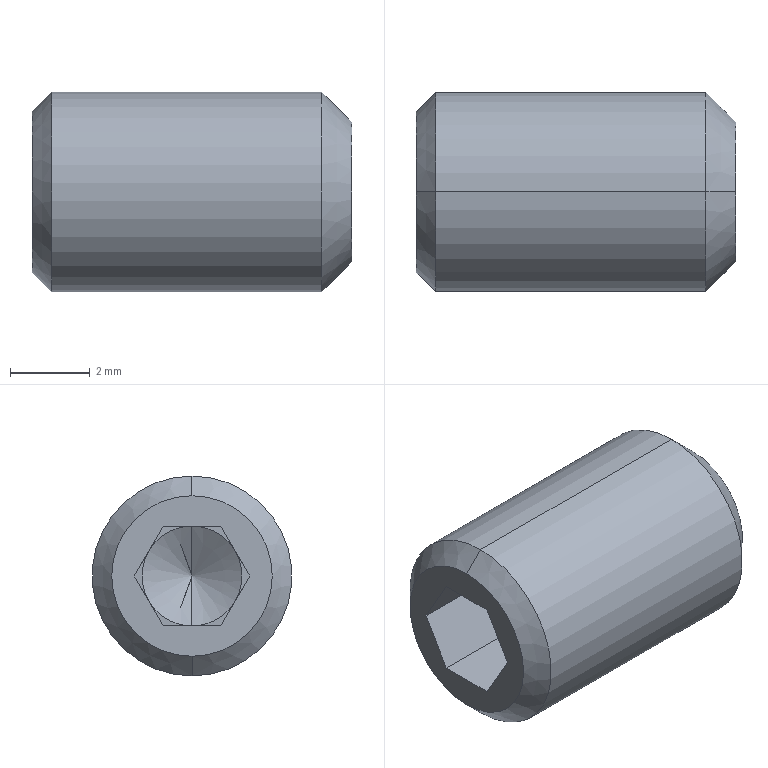Part | STEP file | 0228_305_MSSFS5-8 | 1 solid | 22 faces | box 8 x 5 x 5 mm | volume 139.331 mm3 | plane 14 | cone 6 | cylinder 2 | commonest cylinder face diameters 5 x2
STEP:
#1=CARTESIAN_POINT('',(0.,0.,0.));
#2=DIRECTION('',(0.,0.,1.));
#3=DIRECTION('',(1.,0.,0.));
#4=AXIS2_PLACEMENT_3D('',#1,#2,#3);
#5=CARTESIAN_POINT('',(-3.51,0.,-2.5));
#6=VERTEX_POINT('',#5);
#7=CARTESIAN_POINT('',(-3.51,0.,2.5));
#8=VERTEX_POINT('',#7);
#9=CARTESIAN_POINT('',(-3.51,0.,0.));
#10=DIRECTION('',(1.,0.,0.));
#11=DIRECTION('',(0.,0.,-1.));
#12=AXIS2_PLACEMENT_3D('',#9,#10,#11);
#13=CIRCLE('',#12,2.5);
#14=CARTESIAN_POINT('',(-0.1298,0.,0.));
#15=DIRECTION('',(1.,0.,0.));
#16=DIRECTION('',(0.,0.,-1.));
#17=AXIS2_PLACEMENT_3D('',#14,#15,#16);
#18=CYLINDRICAL_SURFACE('',#17,2.5);
#19=CARTESIAN_POINT('',(0.,-3.38));
#20=DIRECTION('',(1.,0.));
#21=VECTOR('',#20,1.);
#22=LINE('',#19,#21);
#23=(GEOMETRIC_REPRESENTATION_CONTEXT(2)PARAMETRIC_REPRESENTATION_CONTEXT()REPRESENTATION_CONTEXT('',''));
#24=DEFINITIONAL_REPRESENTATION('',(#22),#23);
#25=PCURVE('',#18,#24);
#26=CARTESIAN_POINT('',(-3.51,0.,0.));
#27=DIRECTION('',(1.,0.,0.));
#28=DIRECTION('',(0.,0.,-1.));
#29=AXIS2_PLACEMENT_3D('',#26,#27,#28);
#30=CONICAL_SURFACE('',#29,2.5,0.7854);
#31=CARTESIAN_POINT('',(0.,0.));
#32=DIRECTION('',(1.,0.));
#33=VECTOR('',#32,1.);
#34=LINE('',#31,#33);
#35=(GEOMETRIC_REPRESENTATION_CONTEXT(2)PARAMETRIC_REPRESENTATION_CONTEXT()REPRESENTATION_CONTEXT('',''));
#36=DEFINITIONAL_REPRESENTATION('',(#34),#35);
#37=PCURVE('',#30,#36);
#38=SURFACE_CURVE('',#13,(#25,#37),.PCURVE_S1.);
#39=EDGE_CURVE('',#6,#8,#38,.T.);
#40=ORIENTED_EDGE('',*,*,#39,.T.);
#41=CARTESIAN_POINT('',(3.25,0.,2.5));
#42=VERTEX_POINT('',#41);
#43=CARTESIAN_POINT('',(-0.1298,0.,2.5));
#44=DIRECTION('',(1.,0.,0.));
#45=VECTOR('',#44,1.);
#46=LINE('',#43,#45);
#47=CARTESIAN_POINT('',(3.142,0.));
#48=DIRECTION('',(0.,1.));
#49=VECTOR('',#48,1.);
#50=LINE('',#47,#49);
#51=(GEOMETRIC_REPRESENTATION_CONTEXT(2)PARAMETRIC_REPRESENTATION_CONTEXT()REPRESENTATION_CONTEXT('',''));
#52=DEFINITIONAL_REPRESENTATION('',(#50),#51);
#53=PCURVE('',#18,#52);
#54=CARTESIAN_POINT('',(-0.1298,0.,0.));
#55=DIRECTION('',(1.,0.,0.));
#56=DIRECTION('',(0.,0.,-1.));
#57=AXIS2_PLACEMENT_3D('',#54,#55,#56);
#58=CYLINDRICAL_SURFACE('',#57,2.5);
#59=CARTESIAN_POINT('',(3.142,0.));
#60=DIRECTION('',(0.,1.));
#61=VECTOR('',#60,1.);
#62=LINE('',#59,#61);
#63=(GEOMETRIC_REPRESENTATION_CONTEXT(2)PARAMETRIC_REPRESENTATION_CONTEXT()REPRESENTATION_CONTEXT('',''));
#64=DEFINITIONAL_REPRESENTATION('',(#62),#63);
#65=PCURVE('',#58,#64);
#66=SURFACE_CURVE('',#46,(#53,#65),.PCURVE_S1.);
#67=EDGE_CURVE('',#8,#42,#66,.T.);
#68=ORIENTED_EDGE('',*,*,#67,.T.);
#69=CARTESIAN_POINT('',(3.25,0.,-2.5));
#70=VERTEX_POINT('',#69);
#71=CARTESIAN_POINT('',(3.25,0.,0.));
#72=DIRECTION('',(-1.,0.,0.));
#73=DIRECTION('',(0.,0.,-1.));
#74=AXIS2_PLACEMENT_3D('',#71,#72,#73);
#75=CIRCLE('',#74,2.5);
#76=CARTESIAN_POINT('',(6.283,3.38));
#77=DIRECTION('',(-1.,0.));
#78=VECTOR('',#77,1.);
#79=LINE('',#76,#78);
#80=(GEOMETRIC_REPRESENTATION_CONTEXT(2)PARAMETRIC_REPRESENTATION_CONTEXT()REPRESENTATION_CONTEXT('',''));
#81=DEFINITIONAL_REPRESENTATION('',(#79),#80);
#82=PCURVE('',#18,#81);
#83=CARTESIAN_POINT('',(3.25,0.,0.));
#84=DIRECTION('',(-1.,0.,0.));
#85=DIRECTION('',(0.,0.,1.));
#86=AXIS2_PLACEMENT_3D('',#83,#84,#85);
#87=CONICAL_SURFACE('',#86,2.5,0.7854);
#88=CARTESIAN_POINT('',(-3.142,0.));
#89=DIRECTION('',(1.,0.));
#90=VECTOR('',#89,1.);
#91=LINE('',#88,#90);
#92=(GEOMETRIC_REPRESENTATION_CONTEXT(2)PARAMETRIC_REPRESENTATION_CONTEXT()REPRESENTATION_CONTEXT('',''));
#93=DEFINITIONAL_REPRESENTATION('',(#91),#92);
#94=PCURVE('',#87,#93);
#95=SURFACE_CURVE('',#75,(#82,#94),.PCURVE_S1.);
#96=EDGE_CURVE('',#42,#70,#95,.T.);
#97=ORIENTED_EDGE('',*,*,#96,.T.);
#98=CARTESIAN_POINT('',(-0.1298,0.,-2.5));
#99=DIRECTION('',(1.,0.,0.));
#100=VECTOR('',#99,1.);
#101=LINE('',#98,#100);
#102=CARTESIAN_POINT('',(0.,0.));
#103=DIRECTION('',(0.,1.));
#104=VECTOR('',#103,1.);
#105=LINE('',#102,#104);
#106=(GEOMETRIC_REPRESENTATION_CONTEXT(2)PARAMETRIC_REPRESENTATION_CONTEXT()REPRESENTATION_CONTEXT('',''));
#107=DEFINITIONAL_REPRESENTATION('',(#105),#106);
#108=PCURVE('',#18,#107);
#109=CARTESIAN_POINT('',(6.283,0.));
#110=DIRECTION('',(0.,1.));
#111=VECTOR('',#110,1.);
#112=LINE('',#109,#111);
#113=(GEOMETRIC_REPRESENTATION_CONTEXT(2)PARAMETRIC_REPRESENTATION_CONTEXT()REPRESENTATION_CONTEXT('',''));
#114=DEFINITIONAL_REPRESENTATION('',(#112),#113);
#115=PCURVE('',#58,#114);
#116=SURFACE_CURVE('',#101,(#108,#115),.PCURVE_S1.);
#117=EDGE_CURVE('',#6,#70,#116,.T.);
#118=ORIENTED_EDGE('',*,*,#117,.F.);
#119=EDGE_LOOP('',(#40,#68,#97,#118));
#120=FACE_BOUND('',#119,.T.);
#121=ADVANCED_FACE('',(#120),#18,.T.);
#122=CARTESIAN_POINT('',(-4.,0.,-2.009));
#123=VERTEX_POINT('',#122);
#124=CARTESIAN_POINT('',(-4.,0.,2.009));
#125=VERTEX_POINT('',#124);
#126=CARTESIAN_POINT('',(-4.,0.,0.));
#127=DIRECTION('',(1.,0.,0.));
#128=DIRECTION('',(0.,0.,-1.));
#129=AXIS2_PLACEMENT_3D('',#126,#127,#128);
#130=CIRCLE('',#129,2.009);
#131=CARTESIAN_POINT('',(0.,-0.4905));
#132=DIRECTION('',(1.,0.));
#133=VECTOR('',#132,1.);
#134=LINE('',#131,#133);
#135=(GEOMETRIC_REPRESENTATION_CONTEXT(2)PARAMETRIC_REPRESENTATION_CONTEXT()REPRESENTATION_CONTEXT('',''));
#136=DEFINITIONAL_REPRESENTATION('',(#134),#135);
#137=PCURVE('',#30,#136);
#138=CARTESIAN_POINT('',(-4.,1.005,0.));
#139=DIRECTION('',(-1.,0.,0.));
#140=DIRECTION('',(0.,0.,1.));
#141=AXIS2_PLACEMENT_3D('',#138,#139,#140);
#142=PLANE('',#141);
#143=CARTESIAN_POINT('',(-2.009,-1.005));
#144=CARTESIAN_POINT('',(-2.009,2.476));
#145=CARTESIAN_POINT('',(1.005,0.7355));
#146=CARTESIAN_POINT('',(4.019,-1.005));
#147=CARTESIAN_POINT('',(1.005,-2.745));
#148=CARTESIAN_POINT('',(-2.009,-4.485));
#149=CARTESIAN_POINT('',(-2.009,-1.005));
#150=(BOUNDED_CURVE()B_SPLINE_CURVE(2,(#143,#144,#145,#146,#147,#148,#149),.UNSPECIFIED.,.T.,.F.)B_SPLINE_CURVE_WITH_KNOTS((1,2,2,2,2,1),(-2.094,0.,2.094,4.189,6.283,8.378),.UNSPECIFIED.)CURVE()GEOMETRIC_REPRESENTATION_ITEM()RATIONAL_B_SPLINE_CURVE((1.,0.5,1.,0.5,1.,0.5,1.))REPRESENTATION_ITEM(''));
#151=(GEOMETRIC_REPRESENTATION_CONTEXT(2)PARAMETRIC_REPRESENTATION_CONTEXT()REPRESENTATION_CONTEXT('',''));
#152=DEFINITIONAL_REPRESENTATION('',(#150),#151);
#153=PCURVE('',#142,#152);
#154=SURFACE_CURVE('',#130,(#137,#153),.PCURVE_S1.);
#155=EDGE_CURVE('',#123,#125,#154,.T.);
#156=ORIENTED_EDGE('',*,*,#155,.T.);
#157=CARTESIAN_POINT('',(-3.51,0.,2.5));
#158=DIRECTION('',(0.7071,0.,0.7071));
#159=VECTOR('',#158,1.);
#160=LINE('',#157,#159);
#161=CARTESIAN_POINT('',(3.142,0.));
#162=DIRECTION('',(0.,1.));
#163=VECTOR('',#162,1.);
#164=LINE('',#161,#163);
#165=(GEOMETRIC_REPRESENTATION_CONTEXT(2)PARAMETRIC_REPRESENTATION_CONTEXT()REPRESENTATION_CONTEXT('',''));
#166=DEFINITIONAL_REPRESENTATION('',(#164),#165);
#167=PCURVE('',#30,#166);
#168=CARTESIAN_POINT('',(-3.51,0.,0.));
#169=DIRECTION('',(1.,0.,0.));
#170=DIRECTION('',(0.,0.,-1.));
#171=AXIS2_PLACEMENT_3D('',#168,#169,#170);
#172=CONICAL_SURFACE('',#171,2.5,0.7854);
#173=CARTESIAN_POINT('',(3.142,0.));
#174=DIRECTION('',(0.,1.));
#175=VECTOR('',#174,1.);
#176=LINE('',#173,#175);
#177=(GEOMETRIC_REPRESENTATION_CONTEXT(2)PARAMETRIC_REPRESENTATION_CONTEXT()REPRESENTATION_CONTEXT('',''));
#178=DEFINITIONAL_REPRESENTATION('',(#176),#177);
#179=PCURVE('',#172,#178);
#180=SURFACE_CURVE('',#160,(#167,#179),.PCURVE_S1.);
#181=EDGE_CURVE('',#125,#8,#180,.T.);
#182=ORIENTED_EDGE('',*,*,#181,.T.);
#183=ORIENTED_EDGE('',*,*,#39,.F.);
#184=CARTESIAN_POINT('',(-3.51,0.,-2.5));
#185=DIRECTION('',(0.7071,0.,-0.7071));
#186=VECTOR('',#185,1.);
#187=LINE('',#184,#186);
#188=CARTESIAN_POINT('',(0.,0.));
#189=DIRECTION('',(0.,1.));
#190=VECTOR('',#189,1.);
#191=LINE('',#188,#190);
#192=(GEOMETRIC_REPRESENTATION_CONTEXT(2)PARAMETRIC_REPRESENTATION_CONTEXT()REPRESENTATION_CONTEXT('',''));
#193=DEFINITIONAL_REPRESENTATION('',(#191),#192);
#194=PCURVE('',#30,#193);
#195=CARTESIAN_POINT('',(6.283,0.));
#196=DIRECTION('',(0.,1.));
#197=VECTOR('',#196,1.);
#198=LINE('',#195,#197);
#199=(GEOMETRIC_REPRESENTATION_CONTEXT(2)PARAMETRIC_REPRESENTATION_CONTEXT()REPRESENTATION_CONTEXT('',''));
#200=DEFINITIONAL_REPRESENTATION('',(#198),#199);
#201=PCURVE('',#172,#200);
#202=SURFACE_CURVE('',#187,(#194,#201),.PCURVE_S1.);
#203=EDGE_CURVE('',#123,#6,#202,.T.);
#204=ORIENTED_EDGE('',*,*,#203,.F.);
#205=EDGE_LOOP('',(#156,#182,#183,#204));
#206=FACE_BOUND('',#205,.T.);
#207=ADVANCED_FACE('',(#206),#30,.T.);
#208=CARTESIAN_POINT('',(4.,0.,1.75));
#209=VERTEX_POINT('',#208);
#210=CARTESIAN_POINT('',(4.,0.,-1.75));
#211=VERTEX_POINT('',#210);
#212=CARTESIAN_POINT('',(4.,0.,0.));
#213=DIRECTION('',(-1.,0.,0.));
#214=DIRECTION('',(0.,0.,1.));
#215=AXIS2_PLACEMENT_3D('',#212,#213,#214);
#216=CIRCLE('',#215,1.75);
#217=CARTESIAN_POINT('',(0.,-0.75));
#218=DIRECTION('',(1.,0.));
#219=VECTOR('',#218,1.);
#220=LINE('',#217,#219);
#221=(GEOMETRIC_REPRESENTATION_CONTEXT(2)PARAMETRIC_REPRESENTATION_CONTEXT()REPRESENTATION_CONTEXT('',''));
#222=DEFINITIONAL_REPRESENTATION('',(#220),#221);
#223=PCURVE('',#87,#222);
#224=CARTESIAN_POINT('',(4.,0.875,0.));
#225=DIRECTION('',(1.,0.,0.));
#226=DIRECTION('',(0.,0.,-1.));
#227=AXIS2_PLACEMENT_3D('',#224,#225,#226);
#228=PLANE('',#227);
#229=CARTESIAN_POINT('',(-1.75,-0.875));
#230=CARTESIAN_POINT('',(-1.75,2.156));
#231=CARTESIAN_POINT('',(0.875,0.6405));
#232=CARTESIAN_POINT('',(3.5,-0.875));
#233=CARTESIAN_POINT('',(0.875,-2.391));
#234=CARTESIAN_POINT('',(-1.75,-3.906));
#235=CARTESIAN_POINT('',(-1.75,-0.875));
#236=(BOUNDED_CURVE()B_SPLINE_CURVE(2,(#229,#230,#231,#232,#233,#234,#235),.UNSPECIFIED.,.T.,.F.)B_SPLINE_CURVE_WITH_KNOTS((1,2,2,2,2,1),(-2.094,0.,2.094,4.189,6.283,8.378),.UNSPECIFIED.)CURVE()GEOMETRIC_REPRESENTATION_ITEM()RATIONAL_B_SPLINE_CURVE((1.,0.5,1.,0.5,1.,0.5,1.))REPRESENTATION_ITEM(''));
#237=(GEOMETRIC_REPRESENTATION_CONTEXT(2)PARAMETRIC_REPRESENTATION_CONTEXT()REPRESENTATION_CONTEXT('',''));
#238=DEFINITIONAL_REPRESENTATION('',(#236),#237);
#239=PCURVE('',#228,#238);
#240=SURFACE_CURVE('',#216,(#223,#239),.PCURVE_S1.);
#241=EDGE_CURVE('',#209,#211,#240,.T.);
#242=ORIENTED_EDGE('',*,*,#241,.T.);
#243=CARTESIAN_POINT('',(3.25,0.,-2.5));
#244=DIRECTION('',(-0.7071,0.,-0.7071));
#245=VECTOR('',#244,1.);
#246=LINE('',#243,#245);
#247=CARTESIAN_POINT('',(3.142,0.));
#248=DIRECTION('',(0.,1.));
#249=VECTOR('',#248,1.);
#250=LINE('',#247,#249);
#251=(GEOMETRIC_REPRESENTATION_CONTEXT(2)PARAMETRIC_REPRESENTATION_CONTEXT()REPRESENTATION_CONTEXT('',''));
#252=DEFINITIONAL_REPRESENTATION('',(#250),#251);
#253=PCURVE('',#87,#252);
#254=CARTESIAN_POINT('',(3.25,0.,0.));
#255=DIRECTION('',(-1.,0.,0.));
#256=DIRECTION('',(0.,0.,1.));
#257=AXIS2_PLACEMENT_3D('',#254,#255,#256);
#258=CONICAL_SURFACE('',#257,2.5,0.7854);
#259=CARTESIAN_POINT('',(3.142,0.));
#260=DIRECTION('',(0.,1.));
#261=VECTOR('',#260,1.);
#262=LINE('',#259,#261);
#263=(GEOMETRIC_REPRESENTATION_CONTEXT(2)PARAMETRIC_REPRESENTATION_CONTEXT()REPRESENTATION_CONTEXT('',''));
#264=DEFINITIONAL_REPRESENTATION('',(#262),#263);
#265=PCURVE('',#258,#264);
#266=SURFACE_CURVE('',#246,(#253,#265),.PCURVE_S1.);
#267=EDGE_CURVE('',#211,#70,#266,.T.);
#268=ORIENTED_EDGE('',*,*,#267,.T.);
#269=ORIENTED_EDGE('',*,*,#96,.F.);
#270=CARTESIAN_POINT('',(3.25,0.,2.5));
#271=DIRECTION('',(-0.7071,0.,0.7071));
#272=VECTOR('',#271,1.);
#273=LINE('',#270,#272);
#274=CARTESIAN_POINT('',(0.,0.));
#275=DIRECTION('',(0.,1.));
#276=VECTOR('',#275,1.);
#277=LINE('',#274,#276);
#278=(GEOMETRIC_REPRESENTATION_CONTEXT(2)PARAMETRIC_REPRESENTATION_CONTEXT()REPRESENTATION_CONTEXT('',''));
#279=DEFINITIONAL_REPRESENTATION('',(#277),#278);
#280=PCURVE('',#87,#279);
#281=CARTESIAN_POINT('',(6.283,0.));
#282=DIRECTION('',(0.,1.));
#283=VECTOR('',#282,1.);
#284=LINE('',#281,#283);
#285=(GEOMETRIC_REPRESENTATION_CONTEXT(2)PARAMETRIC_REPRESENTATION_CONTEXT()REPRESENTATION_CONTEXT('',''));
#286=DEFINITIONAL_REPRESENTATION('',(#284),#285);
#287=PCURVE('',#258,#286);
#288=SURFACE_CURVE('',#273,(#280,#287),.PCURVE_S1.);
#289=EDGE_CURVE('',#209,#42,#288,.T.);
#290=ORIENTED_EDGE('',*,*,#289,.F.);
#291=EDGE_LOOP('',(#242,#268,#269,#290));
#292=FACE_BOUND('',#291,.T.);
#293=ADVANCED_FACE('',(#292),#87,.T.);
#294=CARTESIAN_POINT('',(-2.,0.,1.25));
#295=VERTEX_POINT('',#294);
#296=CARTESIAN_POINT('',(-2.,-1.083,0.625));
#297=VERTEX_POINT('',#296);
#298=CARTESIAN_POINT('',(-2.,0.,0.));
#299=DIRECTION('',(1.,0.,0.));
#300=DIRECTION('',(0.,0.,1.));
#301=AXIS2_PLACEMENT_3D('',#298,#299,#300);
#302=CIRCLE('',#301,1.25);
#303=CARTESIAN_POINT('',(-2.,0.,0.));
#304=DIRECTION('',(-1.,0.,0.));
#305=DIRECTION('',(0.,0.,1.));
#306=AXIS2_PLACEMENT_3D('',#303,#304,#305);
#307=CONICAL_SURFACE('',#306,1.25,1.047);
#308=CARTESIAN_POINT('',(6.283,0.));
#309=DIRECTION('',(-1.,0.));
#310=VECTOR('',#309,1.);
#311=LINE('',#308,#310);
#312=(GEOMETRIC_REPRESENTATION_CONTEXT(2)PARAMETRIC_REPRESENTATION_CONTEXT()REPRESENTATION_CONTEXT('',''));
#313=DEFINITIONAL_REPRESENTATION('',(#311),#312);
#314=PCURVE('',#307,#313);
#315=CARTESIAN_POINT('',(-2.,0.,0.));
#316=DIRECTION('',(1.,0.,0.));
#317=DIRECTION('',(0.,0.,-1.));
#318=AXIS2_PLACEMENT_3D('',#315,#316,#317);
#319=PLANE('',#318);
#320=CARTESIAN_POINT('',(0.,0.));
#321=DIRECTION('',(-1.,0.));
#322=AXIS2_PLACEMENT_2D('',#320,#321);
#323=CIRCLE('',#322,1.25);
#324=(GEOMETRIC_REPRESENTATION_CONTEXT(2)PARAMETRIC_REPRESENTATION_CONTEXT()REPRESENTATION_CONTEXT('',''));
#325=DEFINITIONAL_REPRESENTATION('',(#323),#324);
#326=PCURVE('',#319,#325);
#327=SURFACE_CURVE('',#302,(#314,#326),.PCURVE_S1.);
#328=EDGE_CURVE('',#295,#297,#327,.T.);
#329=ORIENTED_EDGE('',*,*,#328,.T.);
#330=CARTESIAN_POINT('',(-2.,-1.083,-0.625));
#331=VERTEX_POINT('',#330);
#332=CARTESIAN_POINT('',(-2.,0.,0.));
#333=DIRECTION('',(1.,0.,0.));
#334=DIRECTION('',(0.,0.,1.));
#335=AXIS2_PLACEMENT_3D('',#332,#333,#334);
#336=CIRCLE('',#335,1.25);
#337=CARTESIAN_POINT('',(6.283,0.));
#338=DIRECTION('',(-1.,0.));
#339=VECTOR('',#338,1.);
#340=LINE('',#337,#339);
#341=(GEOMETRIC_REPRESENTATION_CONTEXT(2)PARAMETRIC_REPRESENTATION_CONTEXT()REPRESENTATION_CONTEXT('',''));
#342=DEFINITIONAL_REPRESENTATION('',(#340),#341);
#343=PCURVE('',#307,#342);
#344=CARTESIAN_POINT('',(-2.,0.,0.));
#345=DIRECTION('',(1.,0.,0.));
#346=DIRECTION('',(0.,0.,-1.));
#347=AXIS2_PLACEMENT_3D('',#344,#345,#346);
#348=PLANE('',#347);
#349=CARTESIAN_POINT('',(0.,0.));
#350=DIRECTION('',(-1.,0.));
#351=AXIS2_PLACEMENT_2D('',#349,#350);
#352=CIRCLE('',#351,1.25);
#353=(GEOMETRIC_REPRESENTATION_CONTEXT(2)PARAMETRIC_REPRESENTATION_CONTEXT()REPRESENTATION_CONTEXT('',''));
#354=DEFINITIONAL_REPRESENTATION('',(#352),#353);
#355=PCURVE('',#348,#354);
#356=SURFACE_CURVE('',#336,(#343,#355),.PCURVE_S1.);
#357=EDGE_CURVE('',#297,#331,#356,.T.);
#358=ORIENTED_EDGE('',*,*,#357,.T.);
#359=CARTESIAN_POINT('',(-2.,0.,-1.25));
#360=VERTEX_POINT('',#359);
#361=CARTESIAN_POINT('',(-2.,0.,0.));
#362=DIRECTION('',(-1.,0.,0.));
#363=DIRECTION('',(0.,0.,1.));
#364=AXIS2_PLACEMENT_3D('',#361,#362,#363);
#365=CIRCLE('',#364,1.25);
#366=CARTESIAN_POINT('',(0.,0.));
#367=DIRECTION('',(1.,0.));
#368=VECTOR('',#367,1.);
#369=LINE('',#366,#368);
#370=(GEOMETRIC_REPRESENTATION_CONTEXT(2)PARAMETRIC_REPRESENTATION_CONTEXT()REPRESENTATION_CONTEXT('',''));
#371=DEFINITIONAL_REPRESENTATION('',(#369),#370);
#372=PCURVE('',#307,#371);
#373=CARTESIAN_POINT('',(-2.,0.,0.));
#374=DIRECTION('',(1.,0.,0.));
#375=DIRECTION('',(0.,0.,-1.));
#376=AXIS2_PLACEMENT_3D('',#373,#374,#375);
#377=PLANE('',#376);
#378=CARTESIAN_POINT('',(-1.25,0.));
#379=CARTESIAN_POINT('',(-1.25,2.165));
#380=CARTESIAN_POINT('',(0.625,1.083));
#381=CARTESIAN_POINT('',(2.5,0.));
#382=CARTESIAN_POINT('',(0.625,-1.083));
#383=CARTESIAN_POINT('',(-1.25,-2.165));
#384=CARTESIAN_POINT('',(-1.25,0.));
#385=(BOUNDED_CURVE()B_SPLINE_CURVE(2,(#378,#379,#380,#381,#382,#383,#384),.UNSPECIFIED.,.T.,.F.)B_SPLINE_CURVE_WITH_KNOTS((1,2,2,2,2,1),(-2.094,0.,2.094,4.189,6.283,8.378),.UNSPECIFIED.)CURVE()GEOMETRIC_REPRESENTATION_ITEM()RATIONAL_B_SPLINE_CURVE((1.,0.5,1.,0.5,1.,0.5,1.))REPRESENTATION_ITEM(''));
#386=(GEOMETRIC_REPRESENTATION_CONTEXT(2)PARAMETRIC_REPRESENTATION_CONTEXT()REPRESENTATION_CONTEXT('',''));
#387=DEFINITIONAL_REPRESENTATION('',(#385),#386);
#388=PCURVE('',#377,#387);
#389=SURFACE_CURVE('',#365,(#372,#388),.PCURVE_S1.);
#390=EDGE_CURVE('',#360,#331,#389,.T.);
#391=ORIENTED_EDGE('',*,*,#390,.F.);
#392=CARTESIAN_POINT('',(-1.278,0.,0.));
#393=VERTEX_POINT('',#392);
#394=CARTESIAN_POINT('',(-2.,0.,-1.25));
#395=DIRECTION('',(-0.5,0.,-0.866));
#396=VECTOR('',#395,1.);
#397=LINE('',#394,#396);
#398=CARTESIAN_POINT('',(3.142,0.));
#399=DIRECTION('',(0.,1.));
#400=VECTOR('',#399,1.);
#401=LINE('',#398,#400);
#402=(GEOMETRIC_REPRESENTATION_CONTEXT(2)PARAMETRIC_REPRESENTATION_CONTEXT()REPRESENTATION_CONTEXT('',''));
#403=DEFINITIONAL_REPRESENTATION('',(#401),#402);
#404=PCURVE('',#307,#403);
#405=CARTESIAN_POINT('',(-2.,0.,0.));
#406=DIRECTION('',(-1.,0.,0.));
#407=DIRECTION('',(0.,0.,1.));
#408=AXIS2_PLACEMENT_3D('',#405,#406,#407);
#409=CONICAL_SURFACE('',#408,1.25,1.047);
#410=CARTESIAN_POINT('',(3.142,0.));
#411=DIRECTION('',(0.,1.));
#412=VECTOR('',#411,1.);
#413=LINE('',#410,#412);
#414=(GEOMETRIC_REPRESENTATION_CONTEXT(2)PARAMETRIC_REPRESENTATION_CONTEXT()REPRESENTATION_CONTEXT('',''));
#415=DEFINITIONAL_REPRESENTATION('',(#413),#414);
#416=PCURVE('',#409,#415);
#417=SURFACE_CURVE('',#397,(#404,#416),.PCURVE_S1.);
#418=EDGE_CURVE('',#393,#360,#417,.T.);
#419=ORIENTED_EDGE('',*,*,#418,.F.);
#420=CARTESIAN_POINT('',(-2.,0.,1.25));
#421=DIRECTION('',(-0.5,0.,0.866));
#422=VECTOR('',#421,1.);
#423=LINE('',#420,#422);
#424=CARTESIAN_POINT('',(6.283,0.));
#425=DIRECTION('',(0.,1.));
#426=VECTOR('',#425,1.);
#427=LINE('',#424,#426);
#428=(GEOMETRIC_REPRESENTATION_CONTEXT(2)PARAMETRIC_REPRESENTATION_CONTEXT()REPRESENTATION_CONTEXT('',''));
#429=DEFINITIONAL_REPRESENTATION('',(#427),#428);
#430=PCURVE('',#307,#429);
#431=CARTESIAN_POINT('',(0.,0.));
#432=DIRECTION('',(0.,1.));
#433=VECTOR('',#432,1.);
#434=LINE('',#431,#433);
#435=(GEOMETRIC_REPRESENTATION_CONTEXT(2)PARAMETRIC_REPRESENTATION_CONTEXT()REPRESENTATION_CONTEXT('',''));
#436=DEFINITIONAL_REPRESENTATION('',(#434),#435);
#437=PCURVE('',#409,#436);
#438=SURFACE_CURVE('',#423,(#430,#437),.PCURVE_S1.);
#439=EDGE_CURVE('',#393,#295,#438,.T.);
#440=ORIENTED_EDGE('',*,*,#439,.T.);
#441=EDGE_LOOP('',(#329,#358,#391,#419,#440));
#442=FACE_BOUND('',#441,.F.);
#443=ADVANCED_FACE('',(#442),#307,.F.);
#444=ORIENTED_EDGE('',*,*,#67,.F.);
#445=CARTESIAN_POINT('',(-3.51,0.,0.));
#446=DIRECTION('',(1.,0.,0.));
#447=DIRECTION('',(0.,0.,-1.));
#448=AXIS2_PLACEMENT_3D('',#445,#446,#447);
#449=CIRCLE('',#448,2.5);
#450=CARTESIAN_POINT('',(0.,-3.38));
#451=DIRECTION('',(1.,0.));
#452=VECTOR('',#451,1.);
#453=LINE('',#450,#452);
#454=(GEOMETRIC_REPRESENTATION_CONTEXT(2)PARAMETRIC_REPRESENTATION_CONTEXT()REPRESENTATION_CONTEXT('',''));
#455=DEFINITIONAL_REPRESENTATION('',(#453),#454);
#456=PCURVE('',#58,#455);
#457=CARTESIAN_POINT('',(0.,0.));
#458=DIRECTION('',(1.,0.));
#459=VECTOR('',#458,1.);
#460=LINE('',#457,#459);
#461=(GEOMETRIC_REPRESENTATION_CONTEXT(2)PARAMETRIC_REPRESENTATION_CONTEXT()REPRESENTATION_CONTEXT('',''));
#462=DEFINITIONAL_REPRESENTATION('',(#460),#461);
#463=PCURVE('',#172,#462);
#464=SURFACE_CURVE('',#449,(#456,#463),.PCURVE_S1.);
#465=EDGE_CURVE('',#8,#6,#464,.T.);
#466=ORIENTED_EDGE('',*,*,#465,.T.);
#467=ORIENTED_EDGE('',*,*,#117,.T.);
#468=CARTESIAN_POINT('',(3.25,0.,0.));
#469=DIRECTION('',(-1.,0.,0.));
#470=DIRECTION('',(0.,0.,-1.));
#471=AXIS2_PLACEMENT_3D('',#468,#469,#470);
#472=CIRCLE('',#471,2.5);
#473=CARTESIAN_POINT('',(6.283,3.38));
#474=DIRECTION('',(-1.,0.));
#475=VECTOR('',#474,1.);
#476=LINE('',#473,#475);
#477=(GEOMETRIC_REPRESENTATION_CONTEXT(2)PARAMETRIC_REPRESENTATION_CONTEXT()REPRESENTATION_CONTEXT('',''));
#478=DEFINITIONAL_REPRESENTATION('',(#476),#477);
#479=PCURVE('',#58,#478);
#480=CARTESIAN_POINT('',(3.142,0.));
#481=DIRECTION('',(1.,0.));
#482=VECTOR('',#481,1.);
#483=LINE('',#480,#482);
#484=(GEOMETRIC_REPRESENTATION_CONTEXT(2)PARAMETRIC_REPRESENTATION_CONTEXT()REPRESENTATION_CONTEXT('',''));
#485=DEFINITIONAL_REPRESENTATION('',(#483),#484);
#486=PCURVE('',#258,#485);
#487=SURFACE_CURVE('',#472,(#479,#486),.PCURVE_S1.);
#488=EDGE_CURVE('',#70,#42,#487,.T.);
#489=ORIENTED_EDGE('',*,*,#488,.T.);
#490=EDGE_LOOP('',(#444,#466,#467,#489));
#491=FACE_BOUND('',#490,.T.);
#492=ADVANCED_FACE('',(#491),#58,.T.);
#493=ORIENTED_EDGE('',*,*,#181,.F.);
#494=CARTESIAN_POINT('',(-4.,0.,0.));
#495=DIRECTION('',(1.,0.,0.));
#496=DIRECTION('',(0.,0.,-1.));
#497=AXIS2_PLACEMENT_3D('',#494,#495,#496);
#498=CIRCLE('',#497,2.009);
#499=CARTESIAN_POINT('',(0.,-0.4905));
#500=DIRECTION('',(1.,0.));
#501=VECTOR('',#500,1.);
#502=LINE('',#499,#501);
#503=(GEOMETRIC_REPRESENTATION_CONTEXT(2)PARAMETRIC_REPRESENTATION_CONTEXT()REPRESENTATION_CONTEXT('',''));
#504=DEFINITIONAL_REPRESENTATION('',(#502),#503);
#505=PCURVE('',#172,#504);
#506=CARTESIAN_POINT('',(-2.009,-1.005));
#507=CARTESIAN_POINT('',(-2.009,2.476));
#508=CARTESIAN_POINT('',(1.005,0.7355));
#509=CARTESIAN_POINT('',(4.019,-1.005));
#510=CARTESIAN_POINT('',(1.005,-2.745));
#511=CARTESIAN_POINT('',(-2.009,-4.485));
#512=CARTESIAN_POINT('',(-2.009,-1.005));
#513=(BOUNDED_CURVE()B_SPLINE_CURVE(2,(#506,#507,#508,#509,#510,#511,#512),.UNSPECIFIED.,.T.,.F.)B_SPLINE_CURVE_WITH_KNOTS((1,2,2,2,2,1),(-2.094,0.,2.094,4.189,6.283,8.378),.UNSPECIFIED.)CURVE()GEOMETRIC_REPRESENTATION_ITEM()RATIONAL_B_SPLINE_CURVE((1.,0.5,1.,0.5,1.,0.5,1.))REPRESENTATION_ITEM(''));
#514=(GEOMETRIC_REPRESENTATION_CONTEXT(2)PARAMETRIC_REPRESENTATION_CONTEXT()REPRESENTATION_CONTEXT('',''));
#515=DEFINITIONAL_REPRESENTATION('',(#513),#514);
#516=PCURVE('',#142,#515);
#517=SURFACE_CURVE('',#498,(#505,#516),.PCURVE_S1.);
#518=EDGE_CURVE('',#125,#123,#517,.T.);
#519=ORIENTED_EDGE('',*,*,#518,.T.);
#520=ORIENTED_EDGE('',*,*,#203,.T.);
#521=ORIENTED_EDGE('',*,*,#465,.F.);
#522=EDGE_LOOP('',(#493,#519,#520,#521));
#523=FACE_BOUND('',#522,.T.);
#524=ADVANCED_FACE('',(#523),#172,.T.);
#525=ORIENTED_EDGE('',*,*,#267,.F.);
#526=CARTESIAN_POINT('',(4.,0.,0.));
#527=DIRECTION('',(-1.,0.,0.));
#528=DIRECTION('',(0.,0.,1.));
#529=AXIS2_PLACEMENT_3D('',#526,#527,#528);
#530=CIRCLE('',#529,1.75);
#531=CARTESIAN_POINT('',(0.,-0.75));
#532=DIRECTION('',(1.,0.));
#533=VECTOR('',#532,1.);
#534=LINE('',#531,#533);
#535=(GEOMETRIC_REPRESENTATION_CONTEXT(2)PARAMETRIC_REPRESENTATION_CONTEXT()REPRESENTATION_CONTEXT('',''));
#536=DEFINITIONAL_REPRESENTATION('',(#534),#535);
#537=PCURVE('',#258,#536);
#538=CARTESIAN_POINT('',(-1.75,-0.875));
#539=CARTESIAN_POINT('',(-1.75,2.156));
#540=CARTESIAN_POINT('',(0.875,0.6405));
#541=CARTESIAN_POINT('',(3.5,-0.875));
#542=CARTESIAN_POINT('',(0.875,-2.391));
#543=CARTESIAN_POINT('',(-1.75,-3.906));
#544=CARTESIAN_POINT('',(-1.75,-0.875));
#545=(BOUNDED_CURVE()B_SPLINE_CURVE(2,(#538,#539,#540,#541,#542,#543,#544),.UNSPECIFIED.,.T.,.F.)B_SPLINE_CURVE_WITH_KNOTS((1,2,2,2,2,1),(-2.094,0.,2.094,4.189,6.283,8.378),.UNSPECIFIED.)CURVE()GEOMETRIC_REPRESENTATION_ITEM()RATIONAL_B_SPLINE_CURVE((1.,0.5,1.,0.5,1.,0.5,1.))REPRESENTATION_ITEM(''));
#546=(GEOMETRIC_REPRESENTATION_CONTEXT(2)PARAMETRIC_REPRESENTATION_CONTEXT()REPRESENTATION_CONTEXT('',''));
#547=DEFINITIONAL_REPRESENTATION('',(#545),#546);
#548=PCURVE('',#228,#547);
#549=SURFACE_CURVE('',#530,(#537,#548),.PCURVE_S1.);
#550=EDGE_CURVE('',#211,#209,#549,.T.);
#551=ORIENTED_EDGE('',*,*,#550,.T.);
#552=ORIENTED_EDGE('',*,*,#289,.T.);
#553=ORIENTED_EDGE('',*,*,#488,.F.);
#554=EDGE_LOOP('',(#525,#551,#552,#553));
#555=FACE_BOUND('',#554,.T.);
#556=ADVANCED_FACE('',(#555),#258,.T.);
#557=ORIENTED_EDGE('',*,*,#155,.F.);
#558=ORIENTED_EDGE('',*,*,#518,.F.);
#559=EDGE_LOOP('',(#557,#558));
#560=FACE_BOUND('',#559,.T.);
#561=CARTESIAN_POINT('',(-4.,-0.7217,-1.25));
#562=VERTEX_POINT('',#561);
#563=CARTESIAN_POINT('',(-4.,0.7217,-1.25));
#564=VERTEX_POINT('',#563);
#565=CARTESIAN_POINT('',(-4.,0.7217,-1.25));
#566=DIRECTION('',(0.,1.,0.));
#567=VECTOR('',#566,1.);
#568=LINE('',#565,#567);
#569=CARTESIAN_POINT('',(-1.25,-0.2831));
#570=DIRECTION('',(0.,1.));
#571=VECTOR('',#570,1.);
#572=LINE('',#569,#571);
#573=(GEOMETRIC_REPRESENTATION_CONTEXT(2)PARAMETRIC_REPRESENTATION_CONTEXT()REPRESENTATION_CONTEXT('',''));
#574=DEFINITIONAL_REPRESENTATION('',(#572),#573);
#575=PCURVE('',#142,#574);
#576=CARTESIAN_POINT('',(-4.,0.7217,-1.25));
#577=DIRECTION('',(0.,0.,-1.));
#578=DIRECTION('',(-1.,0.,0.));
#579=AXIS2_PLACEMENT_3D('',#576,#577,#578);
#580=PLANE('',#579);
#581=CARTESIAN_POINT('',(0.,0.));
#582=DIRECTION('',(0.,1.));
#583=VECTOR('',#582,1.);
#584=LINE('',#581,#583);
#585=(GEOMETRIC_REPRESENTATION_CONTEXT(2)PARAMETRIC_REPRESENTATION_CONTEXT()REPRESENTATION_CONTEXT('',''));
#586=DEFINITIONAL_REPRESENTATION('',(#584),#585);
#587=PCURVE('',#580,#586);
#588=SURFACE_CURVE('',#568,(#575,#587),.PCURVE_S1.);
#589=EDGE_CURVE('',#562,#564,#588,.T.);
#590=ORIENTED_EDGE('',*,*,#589,.T.);
#591=CARTESIAN_POINT('',(-4.,1.443,0.));
#592=VERTEX_POINT('',#591);
#593=CARTESIAN_POINT('',(-4.,0.7217,-1.25));
#594=DIRECTION('',(0.,0.5,0.866));
#595=VECTOR('',#594,1.);
#596=LINE('',#593,#595);
#597=CARTESIAN_POINT('',(-1.25,-0.2831));
#598=DIRECTION('',(0.866,0.5));
#599=VECTOR('',#598,1.);
#600=LINE('',#597,#599);
#601=(GEOMETRIC_REPRESENTATION_CONTEXT(2)PARAMETRIC_REPRESENTATION_CONTEXT()REPRESENTATION_CONTEXT('',''));
#602=DEFINITIONAL_REPRESENTATION('',(#600),#601);
#603=PCURVE('',#142,#602);
#604=CARTESIAN_POINT('',(-4.,1.443,0.));
#605=DIRECTION('',(0.,0.866,-0.5));
#606=DIRECTION('',(0.,0.5,0.866));
#607=AXIS2_PLACEMENT_3D('',#604,#605,#606);
#608=PLANE('',#607);
#609=CARTESIAN_POINT('',(-1.443,0.));
#610=DIRECTION('',(1.,0.));
#611=VECTOR('',#610,1.);
#612=LINE('',#609,#611);
#613=(GEOMETRIC_REPRESENTATION_CONTEXT(2)PARAMETRIC_REPRESENTATION_CONTEXT()REPRESENTATION_CONTEXT('',''));
#614=DEFINITIONAL_REPRESENTATION('',(#612),#613);
#615=PCURVE('',#608,#614);
#616=SURFACE_CURVE('',#596,(#603,#615),.PCURVE_S1.);
#617=EDGE_CURVE('',#564,#592,#616,.T.);
#618=ORIENTED_EDGE('',*,*,#617,.T.);
#619=CARTESIAN_POINT('',(-4.,0.7217,1.25));
#620=VERTEX_POINT('',#619);
#621=CARTESIAN_POINT('',(-4.,0.7217,1.25));
#622=DIRECTION('',(0.,-0.5,0.866));
#623=VECTOR('',#622,1.);
#624=LINE('',#621,#623);
#625=CARTESIAN_POINT('',(1.25,-0.2831));
#626=DIRECTION('',(0.866,-0.5));
#627=VECTOR('',#626,1.);
#628=LINE('',#625,#627);
#629=(GEOMETRIC_REPRESENTATION_CONTEXT(2)PARAMETRIC_REPRESENTATION_CONTEXT()REPRESENTATION_CONTEXT('',''));
#630=DEFINITIONAL_REPRESENTATION('',(#628),#629);
#631=PCURVE('',#142,#630);
#632=CARTESIAN_POINT('',(-4.,0.7217,1.25));
#633=DIRECTION('',(0.,0.866,0.5));
#634=DIRECTION('',(0.,-0.5,0.866));
#635=AXIS2_PLACEMENT_3D('',#632,#633,#634);
#636=PLANE('',#635);
#637=CARTESIAN_POINT('',(0.,0.));
#638=DIRECTION('',(1.,0.));
#639=VECTOR('',#638,1.);
#640=LINE('',#637,#639);
#641=(GEOMETRIC_REPRESENTATION_CONTEXT(2)PARAMETRIC_REPRESENTATION_CONTEXT()REPRESENTATION_CONTEXT('',''));
#642=DEFINITIONAL_REPRESENTATION('',(#640),#641);
#643=PCURVE('',#636,#642);
#644=SURFACE_CURVE('',#624,(#631,#643),.PCURVE_S1.);
#645=EDGE_CURVE('',#592,#620,#644,.T.);
#646=ORIENTED_EDGE('',*,*,#645,.T.);
#647=CARTESIAN_POINT('',(-4.,-0.7217,1.25));
#648=VERTEX_POINT('',#647);
#649=CARTESIAN_POINT('',(-4.,-0.7217,1.25));
#650=DIRECTION('',(0.,-1.,0.));
#651=VECTOR('',#650,1.);
#652=LINE('',#649,#651);
#653=CARTESIAN_POINT('',(1.25,-1.726));
#654=DIRECTION('',(0.,-1.));
#655=VECTOR('',#654,1.);
#656=LINE('',#653,#655);
#657=(GEOMETRIC_REPRESENTATION_CONTEXT(2)PARAMETRIC_REPRESENTATION_CONTEXT()REPRESENTATION_CONTEXT('',''));
#658=DEFINITIONAL_REPRESENTATION('',(#656),#657);
#659=PCURVE('',#142,#658);
#660=CARTESIAN_POINT('',(-4.,-0.7217,1.25));
#661=DIRECTION('',(0.,0.,1.));
#662=DIRECTION('',(1.,0.,0.));
#663=AXIS2_PLACEMENT_3D('',#660,#661,#662);
#664=PLANE('',#663);
#665=CARTESIAN_POINT('',(0.,0.));
#666=DIRECTION('',(0.,-1.));
#667=VECTOR('',#666,1.);
#668=LINE('',#665,#667);
#669=(GEOMETRIC_REPRESENTATION_CONTEXT(2)PARAMETRIC_REPRESENTATION_CONTEXT()REPRESENTATION_CONTEXT('',''));
#670=DEFINITIONAL_REPRESENTATION('',(#668),#669);
#671=PCURVE('',#664,#670);
#672=SURFACE_CURVE('',#652,(#659,#671),.PCURVE_S1.);
#673=EDGE_CURVE('',#620,#648,#672,.T.);
#674=ORIENTED_EDGE('',*,*,#673,.T.);
#675=CARTESIAN_POINT('',(-4.,-1.443,0.));
#676=VERTEX_POINT('',#675);
#677=CARTESIAN_POINT('',(-4.,-1.443,0.));
#678=DIRECTION('',(0.,-0.5,-0.866));
#679=VECTOR('',#678,1.);
#680=LINE('',#677,#679);
#681=CARTESIAN_POINT('',(0.,-2.448));
#682=DIRECTION('',(-0.866,-0.5));
#683=VECTOR('',#682,1.);
#684=LINE('',#681,#683);
#685=(GEOMETRIC_REPRESENTATION_CONTEXT(2)PARAMETRIC_REPRESENTATION_CONTEXT()REPRESENTATION_CONTEXT('',''));
#686=DEFINITIONAL_REPRESENTATION('',(#684),#685);
#687=PCURVE('',#142,#686);
#688=CARTESIAN_POINT('',(-4.,-1.443,0.));
#689=DIRECTION('',(0.,-0.866,0.5));
#690=DIRECTION('',(0.,-0.5,-0.866));
#691=AXIS2_PLACEMENT_3D('',#688,#689,#690);
#692=PLANE('',#691);
#693=CARTESIAN_POINT('',(0.,0.));
#694=DIRECTION('',(1.,0.));
#695=VECTOR('',#694,1.);
#696=LINE('',#693,#695);
#697=(GEOMETRIC_REPRESENTATION_CONTEXT(2)PARAMETRIC_REPRESENTATION_CONTEXT()REPRESENTATION_CONTEXT('',''));
#698=DEFINITIONAL_REPRESENTATION('',(#696),#697);
#699=PCURVE('',#692,#698);
#700=SURFACE_CURVE('',#680,(#687,#699),.PCURVE_S1.);
#701=EDGE_CURVE('',#648,#676,#700,.T.);
#702=ORIENTED_EDGE('',*,*,#701,.T.);
#703=CARTESIAN_POINT('',(-4.,-0.7217,-1.25));
#704=DIRECTION('',(0.,0.5,-0.866));
#705=VECTOR('',#704,1.);
#706=LINE('',#703,#705);
#707=CARTESIAN_POINT('',(-1.25,-1.726));
#708=DIRECTION('',(-0.866,0.5));
#709=VECTOR('',#708,1.);
#710=LINE('',#707,#709);
#711=(GEOMETRIC_REPRESENTATION_CONTEXT(2)PARAMETRIC_REPRESENTATION_CONTEXT()REPRESENTATION_CONTEXT('',''));
#712=DEFINITIONAL_REPRESENTATION('',(#710),#711);
#713=PCURVE('',#142,#712);
#714=CARTESIAN_POINT('',(-4.,-0.7217,-1.25));
#715=DIRECTION('',(0.,-0.866,-0.5));
#716=DIRECTION('',(0.,0.5,-0.866));
#717=AXIS2_PLACEMENT_3D('',#714,#715,#716);
#718=PLANE('',#717);
#719=CARTESIAN_POINT('',(0.,0.));
#720=DIRECTION('',(1.,0.));
#721=VECTOR('',#720,1.);
#722=LINE('',#719,#721);
#723=(GEOMETRIC_REPRESENTATION_CONTEXT(2)PARAMETRIC_REPRESENTATION_CONTEXT()REPRESENTATION_CONTEXT('',''));
#724=DEFINITIONAL_REPRESENTATION('',(#722),#723);
#725=PCURVE('',#718,#724);
#726=SURFACE_CURVE('',#706,(#713,#725),.PCURVE_S1.);
#727=EDGE_CURVE('',#676,#562,#726,.T.);
#728=ORIENTED_EDGE('',*,*,#727,.T.);
#729=EDGE_LOOP('',(#590,#618,#646,#674,#702,#728));
#730=FACE_BOUND('',#729,.T.);
#731=ADVANCED_FACE('',(#560,#730),#142,.T.);
#732=ORIENTED_EDGE('',*,*,#241,.F.);
#733=ORIENTED_EDGE('',*,*,#550,.F.);
#734=EDGE_LOOP('',(#732,#733));
#735=FACE_BOUND('',#734,.T.);
#736=ADVANCED_FACE('',(#735),#228,.T.);
#737=CARTESIAN_POINT('',(-2.,1.443,0.));
#738=VERTEX_POINT('',#737);
#739=CARTESIAN_POINT('',(-4.,1.443,0.));
#740=DIRECTION('',(1.,0.,0.));
#741=VECTOR('',#740,1.);
#742=LINE('',#739,#741);
#743=CARTESIAN_POINT('',(0.,0.));
#744=DIRECTION('',(0.,1.));
#745=VECTOR('',#744,1.);
#746=LINE('',#743,#745);
#747=(GEOMETRIC_REPRESENTATION_CONTEXT(2)PARAMETRIC_REPRESENTATION_CONTEXT()REPRESENTATION_CONTEXT('',''));
#748=DEFINITIONAL_REPRESENTATION('',(#746),#747);
#749=PCURVE('',#608,#748);
#750=CARTESIAN_POINT('',(-1.443,0.));
#751=DIRECTION('',(0.,1.));
#752=VECTOR('',#751,1.);
#753=LINE('',#750,#752);
#754=(GEOMETRIC_REPRESENTATION_CONTEXT(2)PARAMETRIC_REPRESENTATION_CONTEXT()REPRESENTATION_CONTEXT('',''));
#755=DEFINITIONAL_REPRESENTATION('',(#753),#754);
#756=PCURVE('',#636,#755);
#757=SURFACE_CURVE('',#742,(#749,#756),.PCURVE_S1.);
#758=EDGE_CURVE('',#592,#738,#757,.T.);
#759=ORIENTED_EDGE('',*,*,#758,.F.);
#760=ORIENTED_EDGE('',*,*,#617,.F.);
#761=CARTESIAN_POINT('',(-2.,0.7217,-1.25));
#762=VERTEX_POINT('',#761);
#763=CARTESIAN_POINT('',(-4.,0.7217,-1.25));
#764=DIRECTION('',(-1.,0.,0.));
#765=VECTOR('',#764,1.);
#766=LINE('',#763,#765);
#767=CARTESIAN_POINT('',(-1.443,0.));
#768=DIRECTION('',(0.,-1.));
#769=VECTOR('',#768,1.);
#770=LINE('',#767,#769);
#771=(GEOMETRIC_REPRESENTATION_CONTEXT(2)PARAMETRIC_REPRESENTATION_CONTEXT()REPRESENTATION_CONTEXT('',''));
#772=DEFINITIONAL_REPRESENTATION('',(#770),#771);
#773=PCURVE('',#608,#772);
#774=CARTESIAN_POINT('',(0.,0.));
#775=DIRECTION('',(1.,0.));
#776=VECTOR('',#775,1.);
#777=LINE('',#774,#776);
#778=(GEOMETRIC_REPRESENTATION_CONTEXT(2)PARAMETRIC_REPRESENTATION_CONTEXT()REPRESENTATION_CONTEXT('',''));
#779=DEFINITIONAL_REPRESENTATION('',(#777),#778);
#780=PCURVE('',#580,#779);
#781=SURFACE_CURVE('',#766,(#773,#780),.PCURVE_S1.);
#782=EDGE_CURVE('',#762,#564,#781,.T.);
#783=ORIENTED_EDGE('',*,*,#782,.F.);
#784=CARTESIAN_POINT('',(-2.,1.083,-0.625));
#785=VERTEX_POINT('',#784);
#786=CARTESIAN_POINT('',(-2.,1.443,0.));
#787=DIRECTION('',(0.,-0.5,-0.866));
#788=VECTOR('',#787,1.);
#789=LINE('',#786,#788);
#790=CARTESIAN_POINT('',(0.,2.));
#791=DIRECTION('',(-1.,0.));
#792=VECTOR('',#791,1.);
#793=LINE('',#790,#792);
#794=(GEOMETRIC_REPRESENTATION_CONTEXT(2)PARAMETRIC_REPRESENTATION_CONTEXT()REPRESENTATION_CONTEXT('',''));
#795=DEFINITIONAL_REPRESENTATION('',(#793),#794);
#796=PCURVE('',#608,#795);
#797=CARTESIAN_POINT('',(-2.,0.,0.));
#798=DIRECTION('',(1.,0.,0.));
#799=DIRECTION('',(0.,0.,-1.));
#800=AXIS2_PLACEMENT_3D('',#797,#798,#799);
#801=PLANE('',#800);
#802=CARTESIAN_POINT('',(0.,1.443));
#803=DIRECTION('',(0.866,-0.5));
#804=VECTOR('',#803,1.);
#805=LINE('',#802,#804);
#806=(GEOMETRIC_REPRESENTATION_CONTEXT(2)PARAMETRIC_REPRESENTATION_CONTEXT()REPRESENTATION_CONTEXT('',''));
#807=DEFINITIONAL_REPRESENTATION('',(#805),#806);
#808=PCURVE('',#801,#807);
#809=SURFACE_CURVE('',#789,(#796,#808),.PCURVE_S1.);
#810=EDGE_CURVE('',#785,#762,#809,.T.);
#811=ORIENTED_EDGE('',*,*,#810,.F.);
#812=CARTESIAN_POINT('',(-2.,1.443,0.));
#813=DIRECTION('',(0.,-0.5,-0.866));
#814=VECTOR('',#813,1.);
#815=LINE('',#812,#814);
#816=CARTESIAN_POINT('',(0.,2.));
#817=DIRECTION('',(-1.,0.));
#818=VECTOR('',#817,1.);
#819=LINE('',#816,#818);
#820=(GEOMETRIC_REPRESENTATION_CONTEXT(2)PARAMETRIC_REPRESENTATION_CONTEXT()REPRESENTATION_CONTEXT('',''));
#821=DEFINITIONAL_REPRESENTATION('',(#819),#820);
#822=PCURVE('',#608,#821);
#823=CARTESIAN_POINT('',(-2.,0.,0.));
#824=DIRECTION('',(1.,0.,0.));
#825=DIRECTION('',(0.,0.,-1.));
#826=AXIS2_PLACEMENT_3D('',#823,#824,#825);
#827=PLANE('',#826);
#828=CARTESIAN_POINT('',(0.,1.443));
#829=DIRECTION('',(0.866,-0.5));
#830=VECTOR('',#829,1.);
#831=LINE('',#828,#830);
#832=(GEOMETRIC_REPRESENTATION_CONTEXT(2)PARAMETRIC_REPRESENTATION_CONTEXT()REPRESENTATION_CONTEXT('',''));
#833=DEFINITIONAL_REPRESENTATION('',(#831),#832);
#834=PCURVE('',#827,#833);
#835=SURFACE_CURVE('',#815,(#822,#834),.PCURVE_S1.);
#836=EDGE_CURVE('',#738,#785,#835,.T.);
#837=ORIENTED_EDGE('',*,*,#836,.F.);
#838=EDGE_LOOP('',(#759,#760,#783,#811,#837));
#839=FACE_BOUND('',#838,.T.);
#840=ADVANCED_FACE('',(#839),#608,.F.);
#841=CARTESIAN_POINT('',(-2.,1.083,0.625));
#842=VERTEX_POINT('',#841);
#843=CARTESIAN_POINT('',(-2.,0.,0.));
#844=DIRECTION('',(1.,0.,0.));
#845=DIRECTION('',(0.,0.,1.));
#846=AXIS2_PLACEMENT_3D('',#843,#844,#845);
#847=CIRCLE('',#846,1.25);
#848=CARTESIAN_POINT('',(0.,0.));
#849=DIRECTION('',(-1.,0.));
#850=AXIS2_PLACEMENT_2D('',#848,#849);
#851=CIRCLE('',#850,1.25);
#852=(GEOMETRIC_REPRESENTATION_CONTEXT(2)PARAMETRIC_REPRESENTATION_CONTEXT()REPRESENTATION_CONTEXT('',''));
#853=DEFINITIONAL_REPRESENTATION('',(#851),#852);
#854=PCURVE('',#827,#853);
#855=CARTESIAN_POINT('',(6.283,0.));
#856=DIRECTION('',(-1.,0.));
#857=VECTOR('',#856,1.);
#858=LINE('',#855,#857);
#859=(GEOMETRIC_REPRESENTATION_CONTEXT(2)PARAMETRIC_REPRESENTATION_CONTEXT()REPRESENTATION_CONTEXT('',''));
#860=DEFINITIONAL_REPRESENTATION('',(#858),#859);
#861=PCURVE('',#409,#860);
#862=SURFACE_CURVE('',#847,(#854,#861),.PCURVE_S1.);
#863=EDGE_CURVE('',#785,#842,#862,.T.);
#864=ORIENTED_EDGE('',*,*,#863,.T.);
#865=CARTESIAN_POINT('',(-2.,1.443,0.));
#866=DIRECTION('',(0.,-0.5,0.866));
#867=VECTOR('',#866,1.);
#868=LINE('',#865,#867);
#869=CARTESIAN_POINT('',(0.,1.443));
#870=DIRECTION('',(-0.866,-0.5));
#871=VECTOR('',#870,1.);
#872=LINE('',#869,#871);
#873=(GEOMETRIC_REPRESENTATION_CONTEXT(2)PARAMETRIC_REPRESENTATION_CONTEXT()REPRESENTATION_CONTEXT('',''));
#874=DEFINITIONAL_REPRESENTATION('',(#872),#873);
#875=PCURVE('',#827,#874);
#876=CARTESIAN_POINT('',(-1.443,2.));
#877=DIRECTION('',(1.,0.));
#878=VECTOR('',#877,1.);
#879=LINE('',#876,#878);
#880=(GEOMETRIC_REPRESENTATION_CONTEXT(2)PARAMETRIC_REPRESENTATION_CONTEXT()REPRESENTATION_CONTEXT('',''));
#881=DEFINITIONAL_REPRESENTATION('',(#879),#880);
#882=PCURVE('',#636,#881);
#883=SURFACE_CURVE('',#868,(#875,#882),.PCURVE_S1.);
#884=EDGE_CURVE('',#738,#842,#883,.T.);
#885=ORIENTED_EDGE('',*,*,#884,.F.);
#886=ORIENTED_EDGE('',*,*,#836,.T.);
#887=EDGE_LOOP('',(#864,#885,#886));
#888=FACE_BOUND('',#887,.T.);
#889=ADVANCED_FACE('',(#888),#827,.F.);
#890=CARTESIAN_POINT('',(-2.,0.7217,1.25));
#891=VERTEX_POINT('',#890);
#892=CARTESIAN_POINT('',(-4.,0.7217,1.25));
#893=DIRECTION('',(1.,0.,0.));
#894=VECTOR('',#893,1.);
#895=LINE('',#892,#894);
#896=CARTESIAN_POINT('',(0.,0.));
#897=DIRECTION('',(0.,1.));
#898=VECTOR('',#897,1.);
#899=LINE('',#896,#898);
#900=(GEOMETRIC_REPRESENTATION_CONTEXT(2)PARAMETRIC_REPRESENTATION_CONTEXT()REPRESENTATION_CONTEXT('',''));
#901=DEFINITIONAL_REPRESENTATION('',(#899),#900);
#902=PCURVE('',#636,#901);
#903=CARTESIAN_POINT('',(0.,1.443));
#904=DIRECTION('',(1.,0.));
#905=VECTOR('',#904,1.);
#906=LINE('',#903,#905);
#907=(GEOMETRIC_REPRESENTATION_CONTEXT(2)PARAMETRIC_REPRESENTATION_CONTEXT()REPRESENTATION_CONTEXT('',''));
#908=DEFINITIONAL_REPRESENTATION('',(#906),#907);
#909=PCURVE('',#664,#908);
#910=SURFACE_CURVE('',#895,(#902,#909),.PCURVE_S1.);
#911=EDGE_CURVE('',#620,#891,#910,.T.);
#912=ORIENTED_EDGE('',*,*,#911,.F.);
#913=ORIENTED_EDGE('',*,*,#645,.F.);
#914=ORIENTED_EDGE('',*,*,#758,.T.);
#915=ORIENTED_EDGE('',*,*,#884,.T.);
#916=CARTESIAN_POINT('',(-2.,0.7217,1.25));
#917=DIRECTION('',(0.,0.5,-0.866));
#918=VECTOR('',#917,1.);
#919=LINE('',#916,#918);
#920=CARTESIAN_POINT('',(0.,2.));
#921=DIRECTION('',(-1.,0.));
#922=VECTOR('',#921,1.);
#923=LINE('',#920,#922);
#924=(GEOMETRIC_REPRESENTATION_CONTEXT(2)PARAMETRIC_REPRESENTATION_CONTEXT()REPRESENTATION_CONTEXT('',''));
#925=DEFINITIONAL_REPRESENTATION('',(#923),#924);
#926=PCURVE('',#636,#925);
#927=CARTESIAN_POINT('',(-2.,0.,0.));
#928=DIRECTION('',(1.,0.,0.));
#929=DIRECTION('',(0.,0.,-1.));
#930=AXIS2_PLACEMENT_3D('',#927,#928,#929);
#931=PLANE('',#930);
#932=CARTESIAN_POINT('',(-1.25,0.7217));
#933=DIRECTION('',(0.866,0.5));
#934=VECTOR('',#933,1.);
#935=LINE('',#932,#934);
#936=(GEOMETRIC_REPRESENTATION_CONTEXT(2)PARAMETRIC_REPRESENTATION_CONTEXT()REPRESENTATION_CONTEXT('',''));
#937=DEFINITIONAL_REPRESENTATION('',(#935),#936);
#938=PCURVE('',#931,#937);
#939=SURFACE_CURVE('',#919,(#926,#938),.PCURVE_S1.);
#940=EDGE_CURVE('',#891,#842,#939,.T.);
#941=ORIENTED_EDGE('',*,*,#940,.F.);
#942=EDGE_LOOP('',(#912,#913,#914,#915,#941));
#943=FACE_BOUND('',#942,.T.);
#944=ADVANCED_FACE('',(#943),#636,.F.);
#945=ORIENTED_EDGE('',*,*,#782,.T.);
#946=ORIENTED_EDGE('',*,*,#589,.F.);
#947=CARTESIAN_POINT('',(-2.,-0.7217,-1.25));
#948=VERTEX_POINT('',#947);
#949=CARTESIAN_POINT('',(-4.,-0.7217,-1.25));
#950=DIRECTION('',(-1.,0.,0.));
#951=VECTOR('',#950,1.);
#952=LINE('',#949,#951);
#953=CARTESIAN_POINT('',(0.,-1.443));
#954=DIRECTION('',(1.,0.));
#955=VECTOR('',#954,1.);
#956=LINE('',#953,#955);
#957=(GEOMETRIC_REPRESENTATION_CONTEXT(2)PARAMETRIC_REPRESENTATION_CONTEXT()REPRESENTATION_CONTEXT('',''));
#958=DEFINITIONAL_REPRESENTATION('',(#956),#957);
#959=PCURVE('',#580,#958);
#960=CARTESIAN_POINT('',(0.,0.));
#961=DIRECTION('',(0.,-1.));
#962=VECTOR('',#961,1.);
#963=LINE('',#960,#962);
#964=(GEOMETRIC_REPRESENTATION_CONTEXT(2)PARAMETRIC_REPRESENTATION_CONTEXT()REPRESENTATION_CONTEXT('',''));
#965=DEFINITIONAL_REPRESENTATION('',(#963),#964);
#966=PCURVE('',#718,#965);
#967=SURFACE_CURVE('',#952,(#959,#966),.PCURVE_S1.);
#968=EDGE_CURVE('',#948,#562,#967,.T.);
#969=ORIENTED_EDGE('',*,*,#968,.F.);
#970=CARTESIAN_POINT('',(-2.,0.7217,-1.25));
#971=DIRECTION('',(0.,-1.,0.));
#972=VECTOR('',#971,1.);
#973=LINE('',#970,#972);
#974=CARTESIAN_POINT('',(-2.,0.));
#975=DIRECTION('',(0.,-1.));
#976=VECTOR('',#975,1.);
#977=LINE('',#974,#976);
#978=(GEOMETRIC_REPRESENTATION_CONTEXT(2)PARAMETRIC_REPRESENTATION_CONTEXT()REPRESENTATION_CONTEXT('',''));
#979=DEFINITIONAL_REPRESENTATION('',(#977),#978);
#980=PCURVE('',#580,#979);
#981=CARTESIAN_POINT('',(1.25,0.7217));
#982=DIRECTION('',(0.,-1.));
#983=VECTOR('',#982,1.);
#984=LINE('',#981,#983);
#985=(GEOMETRIC_REPRESENTATION_CONTEXT(2)PARAMETRIC_REPRESENTATION_CONTEXT()REPRESENTATION_CONTEXT('',''));
#986=DEFINITIONAL_REPRESENTATION('',(#984),#985);
#987=PCURVE('',#377,#986);
#988=SURFACE_CURVE('',#973,(#980,#987),.PCURVE_S1.);
#989=EDGE_CURVE('',#360,#948,#988,.T.);
#990=ORIENTED_EDGE('',*,*,#989,.F.);
#991=CARTESIAN_POINT('',(-2.,0.7217,-1.25));
#992=DIRECTION('',(0.,-1.,0.));
#993=VECTOR('',#992,1.);
#994=LINE('',#991,#993);
#995=CARTESIAN_POINT('',(-2.,0.));
#996=DIRECTION('',(0.,-1.));
#997=VECTOR('',#996,1.);
#998=LINE('',#995,#997);
#999=(GEOMETRIC_REPRESENTATION_CONTEXT(2)PARAMETRIC_REPRESENTATION_CONTEXT()REPRESENTATION_CONTEXT('',''));
#1000=DEFINITIONAL_REPRESENTATION('',(#998),#999);
#1001=PCURVE('',#580,#1000);
#1002=CARTESIAN_POINT('',(1.25,0.7217));
#1003=DIRECTION('',(0.,-1.));
#1004=VECTOR('',#1003,1.);
#1005=LINE('',#1002,#1004);
#1006=(GEOMETRIC_REPRESENTATION_CONTEXT(2)PARAMETRIC_REPRESENTATION_CONTEXT()REPRESENTATION_CONTEXT('',''));
#1007=DEFINITIONAL_REPRESENTATION('',(#1005),#1006);
#1008=PCURVE('',#801,#1007);
#1009=SURFACE_CURVE('',#994,(#1001,#1008),.PCURVE_S1.);
#1010=EDGE_CURVE('',#762,#360,#1009,.T.);
#1011=ORIENTED_EDGE('',*,*,#1010,.F.);
#1012=EDGE_LOOP('',(#945,#946,#969,#990,#1011));
#1013=FACE_BOUND('',#1012,.T.);
#1014=ADVANCED_FACE('',(#1013),#580,.F.);
#1015=ORIENTED_EDGE('',*,*,#810,.T.);
#1016=ORIENTED_EDGE('',*,*,#1010,.T.);
#1017=CARTESIAN_POINT('',(-2.,0.,0.));
#1018=DIRECTION('',(-1.,0.,0.));
#1019=DIRECTION('',(0.,0.,1.));
#1020=AXIS2_PLACEMENT_3D('',#1017,#1018,#1019);
#1021=CIRCLE('',#1020,1.25);
#1022=CARTESIAN_POINT('',(-1.25,0.));
#1023=CARTESIAN_POINT('',(-1.25,2.165));
#1024=CARTESIAN_POINT('',(0.625,1.083));
#1025=CARTESIAN_POINT('',(2.5,0.));
#1026=CARTESIAN_POINT('',(0.625,-1.083));
#1027=CARTESIAN_POINT('',(-1.25,-2.165));
#1028=CARTESIAN_POINT('',(-1.25,0.));
#1029=(BOUNDED_CURVE()B_SPLINE_CURVE(2,(#1022,#1023,#1024,#1025,#1026,#1027,#1028),.UNSPECIFIED.,.T.,.F.)B_SPLINE_CURVE_WITH_KNOTS((1,2,2,2,2,1),(-2.094,0.,2.094,4.189,6.283,8.378),.UNSPECIFIED.)CURVE()GEOMETRIC_REPRESENTATION_ITEM()RATIONAL_B_SPLINE_CURVE((1.,0.5,1.,0.5,1.,0.5,1.))REPRESENTATION_ITEM(''));
#1030=(GEOMETRIC_REPRESENTATION_CONTEXT(2)PARAMETRIC_REPRESENTATION_CONTEXT()REPRESENTATION_CONTEXT('',''));
#1031=DEFINITIONAL_REPRESENTATION('',(#1029),#1030);
#1032=PCURVE('',#801,#1031);
#1033=CARTESIAN_POINT('',(0.,0.));
#1034=DIRECTION('',(1.,0.));
#1035=VECTOR('',#1034,1.);
#1036=LINE('',#1033,#1035);
#1037=(GEOMETRIC_REPRESENTATION_CONTEXT(2)PARAMETRIC_REPRESENTATION_CONTEXT()REPRESENTATION_CONTEXT('',''));
#1038=DEFINITIONAL_REPRESENTATION('',(#1036),#1037);
#1039=PCURVE('',#409,#1038);
#1040=SURFACE_CURVE('',#1021,(#1032,#1039),.PCURVE_S1.);
#1041=EDGE_CURVE('',#785,#360,#1040,.T.);
#1042=ORIENTED_EDGE('',*,*,#1041,.F.);
#1043=EDGE_LOOP('',(#1015,#1016,#1042));
#1044=FACE_BOUND('',#1043,.T.);
#1045=ADVANCED_FACE('',(#1044),#801,.F.);
#1046=CARTESIAN_POINT('',(-2.,0.,1.25));
#1047=DIRECTION('',(0.,-1.,0.));
#1048=VECTOR('',#1047,1.);
#1049=LINE('',#1046,#1048);
#1050=CARTESIAN_POINT('',(-1.25,0.));
#1051=DIRECTION('',(0.,-1.));
#1052=VECTOR('',#1051,1.);
#1053=LINE('',#1050,#1052);
#1054=(GEOMETRIC_REPRESENTATION_CONTEXT(2)PARAMETRIC_REPRESENTATION_CONTEXT()REPRESENTATION_CONTEXT('',''));
#1055=DEFINITIONAL_REPRESENTATION('',(#1053),#1054);
#1056=PCURVE('',#931,#1055);
#1057=CARTESIAN_POINT('',(2.,0.7217));
#1058=DIRECTION('',(0.,-1.));
#1059=VECTOR('',#1058,1.);
#1060=LINE('',#1057,#1059);
#1061=(GEOMETRIC_REPRESENTATION_CONTEXT(2)PARAMETRIC_REPRESENTATION_CONTEXT()REPRESENTATION_CONTEXT('',''));
#1062=DEFINITIONAL_REPRESENTATION('',(#1060),#1061);
#1063=PCURVE('',#664,#1062);
#1064=SURFACE_CURVE('',#1049,(#1056,#1063),.PCURVE_S1.);
#1065=EDGE_CURVE('',#891,#295,#1064,.T.);
#1066=ORIENTED_EDGE('',*,*,#1065,.F.);
#1067=ORIENTED_EDGE('',*,*,#940,.T.);
#1068=CARTESIAN_POINT('',(-2.,0.,0.));
#1069=DIRECTION('',(-1.,0.,0.));
#1070=DIRECTION('',(0.,0.,1.));
#1071=AXIS2_PLACEMENT_3D('',#1068,#1069,#1070);
#1072=CIRCLE('',#1071,1.25);
#1073=CARTESIAN_POINT('',(-1.25,0.));
#1074=CARTESIAN_POINT('',(-1.25,2.165));
#1075=CARTESIAN_POINT('',(0.625,1.083));
#1076=CARTESIAN_POINT('',(2.5,0.));
#1077=CARTESIAN_POINT('',(0.625,-1.083));
#1078=CARTESIAN_POINT('',(-1.25,-2.165));
#1079=CARTESIAN_POINT('',(-1.25,0.));
#1080=(BOUNDED_CURVE()B_SPLINE_CURVE(2,(#1073,#1074,#1075,#1076,#1077,#1078,#1079),.UNSPECIFIED.,.T.,.F.)B_SPLINE_CURVE_WITH_KNOTS((1,2,2,2,2,1),(-2.094,0.,2.094,4.189,6.283,8.378),.UNSPECIFIED.)CURVE()GEOMETRIC_REPRESENTATION_ITEM()RATIONAL_B_SPLINE_CURVE((1.,0.5,1.,0.5,1.,0.5,1.))REPRESENTATION_ITEM(''));
#1081=(GEOMETRIC_REPRESENTATION_CONTEXT(2)PARAMETRIC_REPRESENTATION_CONTEXT()REPRESENTATION_CONTEXT('',''));
#1082=DEFINITIONAL_REPRESENTATION('',(#1080),#1081);
#1083=PCURVE('',#931,#1082);
#1084=CARTESIAN_POINT('',(0.,0.));
#1085=DIRECTION('',(1.,0.));
#1086=VECTOR('',#1085,1.);
#1087=LINE('',#1084,#1086);
#1088=(GEOMETRIC_REPRESENTATION_CONTEXT(2)PARAMETRIC_REPRESENTATION_CONTEXT()REPRESENTATION_CONTEXT('',''));
#1089=DEFINITIONAL_REPRESENTATION('',(#1087),#1088);
#1090=PCURVE('',#409,#1089);
#1091=SURFACE_CURVE('',#1072,(#1083,#1090),.PCURVE_S1.);
#1092=EDGE_CURVE('',#295,#842,#1091,.T.);
#1093=ORIENTED_EDGE('',*,*,#1092,.F.);
#1094=EDGE_LOOP('',(#1066,#1067,#1093));
#1095=FACE_BOUND('',#1094,.T.);
#1096=ADVANCED_FACE('',(#1095),#931,.F.);
#1097=CARTESIAN_POINT('',(-2.,-0.7217,1.25));
#1098=VERTEX_POINT('',#1097);
#1099=CARTESIAN_POINT('',(-4.,-0.7217,1.25));
#1100=DIRECTION('',(1.,0.,0.));
#1101=VECTOR('',#1100,1.);
#1102=LINE('',#1099,#1101);
#1103=CARTESIAN_POINT('',(0.,0.));
#1104=DIRECTION('',(1.,0.));
#1105=VECTOR('',#1104,1.);
#1106=LINE('',#1103,#1105);
#1107=(GEOMETRIC_REPRESENTATION_CONTEXT(2)PARAMETRIC_REPRESENTATION_CONTEXT()REPRESENTATION_CONTEXT('',''));
#1108=DEFINITIONAL_REPRESENTATION('',(#1106),#1107);
#1109=PCURVE('',#664,#1108);
#1110=CARTESIAN_POINT('',(-1.443,0.));
#1111=DIRECTION('',(0.,1.));
#1112=VECTOR('',#1111,1.);
#1113=LINE('',#1110,#1112);
#1114=(GEOMETRIC_REPRESENTATION_CONTEXT(2)PARAMETRIC_REPRESENTATION_CONTEXT()REPRESENTATION_CONTEXT('',''));
#1115=DEFINITIONAL_REPRESENTATION('',(#1113),#1114);
#1116=PCURVE('',#692,#1115);
#1117=SURFACE_CURVE('',#1102,(#1109,#1116),.PCURVE_S1.);
#1118=EDGE_CURVE('',#648,#1098,#1117,.T.);
#1119=ORIENTED_EDGE('',*,*,#1118,.F.);
#1120=ORIENTED_EDGE('',*,*,#673,.F.);
#1121=ORIENTED_EDGE('',*,*,#911,.T.);
#1122=ORIENTED_EDGE('',*,*,#1065,.T.);
#1123=CARTESIAN_POINT('',(-2.,-0.7217,1.25));
#1124=DIRECTION('',(0.,1.,0.));
#1125=VECTOR('',#1124,1.);
#1126=LINE('',#1123,#1125);
#1127=CARTESIAN_POINT('',(2.,0.));
#1128=DIRECTION('',(0.,1.));
#1129=VECTOR('',#1128,1.);
#1130=LINE('',#1127,#1129);
#1131=(GEOMETRIC_REPRESENTATION_CONTEXT(2)PARAMETRIC_REPRESENTATION_CONTEXT()REPRESENTATION_CONTEXT('',''));
#1132=DEFINITIONAL_REPRESENTATION('',(#1130),#1131);
#1133=PCURVE('',#664,#1132);
#1134=CARTESIAN_POINT('',(-1.25,-0.7217));
#1135=DIRECTION('',(0.,1.));
#1136=VECTOR('',#1135,1.);
#1137=LINE('',#1134,#1136);
#1138=(GEOMETRIC_REPRESENTATION_CONTEXT(2)PARAMETRIC_REPRESENTATION_CONTEXT()REPRESENTATION_CONTEXT('',''));
#1139=DEFINITIONAL_REPRESENTATION('',(#1137),#1138);
#1140=PCURVE('',#319,#1139);
#1141=SURFACE_CURVE('',#1126,(#1133,#1140),.PCURVE_S1.);
#1142=EDGE_CURVE('',#1098,#295,#1141,.T.);
#1143=ORIENTED_EDGE('',*,*,#1142,.F.);
#1144=EDGE_LOOP('',(#1119,#1120,#1121,#1122,#1143));
#1145=FACE_BOUND('',#1144,.T.);
#1146=ADVANCED_FACE('',(#1145),#664,.F.);
#1147=ORIENTED_EDGE('',*,*,#968,.T.);
#1148=ORIENTED_EDGE('',*,*,#727,.F.);
#1149=CARTESIAN_POINT('',(-2.,-1.443,0.));
#1150=VERTEX_POINT('',#1149);
#1151=CARTESIAN_POINT('',(-4.,-1.443,0.));
#1152=DIRECTION('',(-1.,0.,0.));
#1153=VECTOR('',#1152,1.);
#1154=LINE('',#1151,#1153);
#1155=CARTESIAN_POINT('',(-1.443,0.));
#1156=DIRECTION('',(0.,-1.));
#1157=VECTOR('',#1156,1.);
#1158=LINE('',#1155,#1157);
#1159=(GEOMETRIC_REPRESENTATION_CONTEXT(2)PARAMETRIC_REPRESENTATION_CONTEXT()REPRESENTATION_CONTEXT('',''));
#1160=DEFINITIONAL_REPRESENTATION('',(#1158),#1159);
#1161=PCURVE('',#718,#1160);
#1162=CARTESIAN_POINT('',(0.,0.));
#1163=DIRECTION('',(0.,-1.));
#1164=VECTOR('',#1163,1.);
#1165=LINE('',#1162,#1164);
#1166=(GEOMETRIC_REPRESENTATION_CONTEXT(2)PARAMETRIC_REPRESENTATION_CONTEXT()REPRESENTATION_CONTEXT('',''));
#1167=DEFINITIONAL_REPRESENTATION('',(#1165),#1166);
#1168=PCURVE('',#692,#1167);
#1169=SURFACE_CURVE('',#1154,(#1161,#1168),.PCURVE_S1.);
#1170=EDGE_CURVE('',#1150,#676,#1169,.T.);
#1171=ORIENTED_EDGE('',*,*,#1170,.F.);
#1172=CARTESIAN_POINT('',(-2.,-0.7217,-1.25));
#1173=DIRECTION('',(0.,-0.5,0.866));
#1174=VECTOR('',#1173,1.);
#1175=LINE('',#1172,#1174);
#1176=CARTESIAN_POINT('',(0.,2.));
#1177=DIRECTION('',(-1.,0.));
#1178=VECTOR('',#1177,1.);
#1179=LINE('',#1176,#1178);
#1180=(GEOMETRIC_REPRESENTATION_CONTEXT(2)PARAMETRIC_REPRESENTATION_CONTEXT()REPRESENTATION_CONTEXT('',''));
#1181=DEFINITIONAL_REPRESENTATION('',(#1179),#1180);
#1182=PCURVE('',#718,#1181);
#1183=CARTESIAN_POINT('',(1.25,-0.7217));
#1184=DIRECTION('',(-0.866,-0.5));
#1185=VECTOR('',#1184,1.);
#1186=LINE('',#1183,#1185);
#1187=(GEOMETRIC_REPRESENTATION_CONTEXT(2)PARAMETRIC_REPRESENTATION_CONTEXT()REPRESENTATION_CONTEXT('',''));
#1188=DEFINITIONAL_REPRESENTATION('',(#1186),#1187);
#1189=PCURVE('',#348,#1188);
#1190=SURFACE_CURVE('',#1175,(#1182,#1189),.PCURVE_S1.);
#1191=EDGE_CURVE('',#331,#1150,#1190,.T.);
#1192=ORIENTED_EDGE('',*,*,#1191,.F.);
#1193=CARTESIAN_POINT('',(-2.,-0.7217,-1.25));
#1194=DIRECTION('',(0.,-0.5,0.866));
#1195=VECTOR('',#1194,1.);
#1196=LINE('',#1193,#1195);
#1197=CARTESIAN_POINT('',(0.,2.));
#1198=DIRECTION('',(-1.,0.));
#1199=VECTOR('',#1198,1.);
#1200=LINE('',#1197,#1199);
#1201=(GEOMETRIC_REPRESENTATION_CONTEXT(2)PARAMETRIC_REPRESENTATION_CONTEXT()REPRESENTATION_CONTEXT('',''));
#1202=DEFINITIONAL_REPRESENTATION('',(#1200),#1201);
#1203=PCURVE('',#718,#1202);
#1204=CARTESIAN_POINT('',(1.25,-0.7217));
#1205=DIRECTION('',(-0.866,-0.5));
#1206=VECTOR('',#1205,1.);
#1207=LINE('',#1204,#1206);
#1208=(GEOMETRIC_REPRESENTATION_CONTEXT(2)PARAMETRIC_REPRESENTATION_CONTEXT()REPRESENTATION_CONTEXT('',''));
#1209=DEFINITIONAL_REPRESENTATION('',(#1207),#1208);
#1210=PCURVE('',#377,#1209);
#1211=SURFACE_CURVE('',#1196,(#1203,#1210),.PCURVE_S1.);
#1212=EDGE_CURVE('',#948,#331,#1211,.T.);
#1213=ORIENTED_EDGE('',*,*,#1212,.F.);
#1214=EDGE_LOOP('',(#1147,#1148,#1171,#1192,#1213));
#1215=FACE_BOUND('',#1214,.T.);
#1216=ADVANCED_FACE('',(#1215),#718,.F.);
#1217=ORIENTED_EDGE('',*,*,#989,.T.);
#1218=ORIENTED_EDGE('',*,*,#1212,.T.);
#1219=ORIENTED_EDGE('',*,*,#390,.F.);
#1220=EDGE_LOOP('',(#1217,#1218,#1219));
#1221=FACE_BOUND('',#1220,.T.);
#1222=ADVANCED_FACE('',(#1221),#377,.F.);
#1223=ORIENTED_EDGE('',*,*,#1041,.F.);
#1224=ORIENTED_EDGE('',*,*,#863,.T.);
#1225=ORIENTED_EDGE('',*,*,#1092,.F.);
#1226=ORIENTED_EDGE('',*,*,#439,.F.);
#1227=ORIENTED_EDGE('',*,*,#418,.T.);
#1228=EDGE_LOOP('',(#1223,#1224,#1225,#1226,#1227));
#1229=FACE_BOUND('',#1228,.F.);
#1230=ADVANCED_FACE('',(#1229),#409,.F.);
#1231=CARTESIAN_POINT('',(-2.,-0.7217,1.25));
#1232=DIRECTION('',(0.,-0.5,-0.866));
#1233=VECTOR('',#1232,1.);
#1234=LINE('',#1231,#1233);
#1235=CARTESIAN_POINT('',(-1.25,-0.7217));
#1236=DIRECTION('',(0.866,-0.5));
#1237=VECTOR('',#1236,1.);
#1238=LINE('',#1235,#1237);
#1239=(GEOMETRIC_REPRESENTATION_CONTEXT(2)PARAMETRIC_REPRESENTATION_CONTEXT()REPRESENTATION_CONTEXT('',''));
#1240=DEFINITIONAL_REPRESENTATION('',(#1238),#1239);
#1241=PCURVE('',#319,#1240);
#1242=CARTESIAN_POINT('',(-1.443,2.));
#1243=DIRECTION('',(1.,0.));
#1244=VECTOR('',#1243,1.);
#1245=LINE('',#1242,#1244);
#1246=(GEOMETRIC_REPRESENTATION_CONTEXT(2)PARAMETRIC_REPRESENTATION_CONTEXT()REPRESENTATION_CONTEXT('',''));
#1247=DEFINITIONAL_REPRESENTATION('',(#1245),#1246);
#1248=PCURVE('',#692,#1247);
#1249=SURFACE_CURVE('',#1234,(#1241,#1248),.PCURVE_S1.);
#1250=EDGE_CURVE('',#1098,#297,#1249,.T.);
#1251=ORIENTED_EDGE('',*,*,#1250,.F.);
#1252=ORIENTED_EDGE('',*,*,#1142,.T.);
#1253=ORIENTED_EDGE('',*,*,#328,.T.);
#1254=EDGE_LOOP('',(#1251,#1252,#1253));
#1255=FACE_BOUND('',#1254,.T.);
#1256=ADVANCED_FACE('',(#1255),#319,.F.);
#1257=ORIENTED_EDGE('',*,*,#1170,.T.);
#1258=ORIENTED_EDGE('',*,*,#701,.F.);
#1259=ORIENTED_EDGE('',*,*,#1118,.T.);
#1260=ORIENTED_EDGE('',*,*,#1250,.T.);
#1261=CARTESIAN_POINT('',(-2.,-1.443,0.));
#1262=DIRECTION('',(0.,0.5,0.866));
#1263=VECTOR('',#1262,1.);
#1264=LINE('',#1261,#1263);
#1265=CARTESIAN_POINT('',(0.,2.));
#1266=DIRECTION('',(-1.,0.));
#1267=VECTOR('',#1266,1.);
#1268=LINE('',#1265,#1267);
#1269=(GEOMETRIC_REPRESENTATION_CONTEXT(2)PARAMETRIC_REPRESENTATION_CONTEXT()REPRESENTATION_CONTEXT('',''));
#1270=DEFINITIONAL_REPRESENTATION('',(#1268),#1269);
#1271=PCURVE('',#692,#1270);
#1272=CARTESIAN_POINT('',(0.,-1.443));
#1273=DIRECTION('',(-0.866,0.5));
#1274=VECTOR('',#1273,1.);
#1275=LINE('',#1272,#1274);
#1276=(GEOMETRIC_REPRESENTATION_CONTEXT(2)PARAMETRIC_REPRESENTATION_CONTEXT()REPRESENTATION_CONTEXT('',''));
#1277=DEFINITIONAL_REPRESENTATION('',(#1275),#1276);
#1278=PCURVE('',#348,#1277);
#1279=SURFACE_CURVE('',#1264,(#1271,#1278),.PCURVE_S1.);
#1280=EDGE_CURVE('',#1150,#297,#1279,.T.);
#1281=ORIENTED_EDGE('',*,*,#1280,.F.);
#1282=EDGE_LOOP('',(#1257,#1258,#1259,#1260,#1281));
#1283=FACE_BOUND('',#1282,.T.);
#1284=ADVANCED_FACE('',(#1283),#692,.F.);
#1285=ORIENTED_EDGE('',*,*,#357,.T.);
#1286=ORIENTED_EDGE('',*,*,#1191,.T.);
#1287=ORIENTED_EDGE('',*,*,#1280,.T.);
#1288=EDGE_LOOP('',(#1285,#1286,#1287));
#1289=FACE_BOUND('',#1288,.T.);
#1290=ADVANCED_FACE('',(#1289),#348,.F.);
#1291=CLOSED_SHELL('',(#121,#207,#293,#443,#492,#524,#556,#731,#736,#840,#889,#944,#1014,#1045,#1096,#1146,#1216,#1222,#1230,#1256,#1284,#1290));
#1292=MANIFOLD_SOLID_BREP('',#1291);
#1293=(LENGTH_UNIT()NAMED_UNIT(*)SI_UNIT(.MILLI.,.METRE.));
#1294=UNCERTAINTY_MEASURE_WITH_UNIT(LENGTH_MEASURE(0.0000001),#1293,'','');
#1295=(NAMED_UNIT(*)PLANE_ANGLE_UNIT()SI_UNIT($,.RADIAN.));
#1296=(NAMED_UNIT(*)SI_UNIT($,.STERADIAN.)SOLID_ANGLE_UNIT());
#1297=(GEOMETRIC_REPRESENTATION_CONTEXT(3)GLOBAL_UNCERTAINTY_ASSIGNED_CONTEXT((#1294))GLOBAL_UNIT_ASSIGNED_CONTEXT((#1293,#1295,#1296))REPRESENTATION_CONTEXT('',''));
#1298=ADVANCED_BREP_SHAPE_REPRESENTATION('',(#4,#1292),#1297);